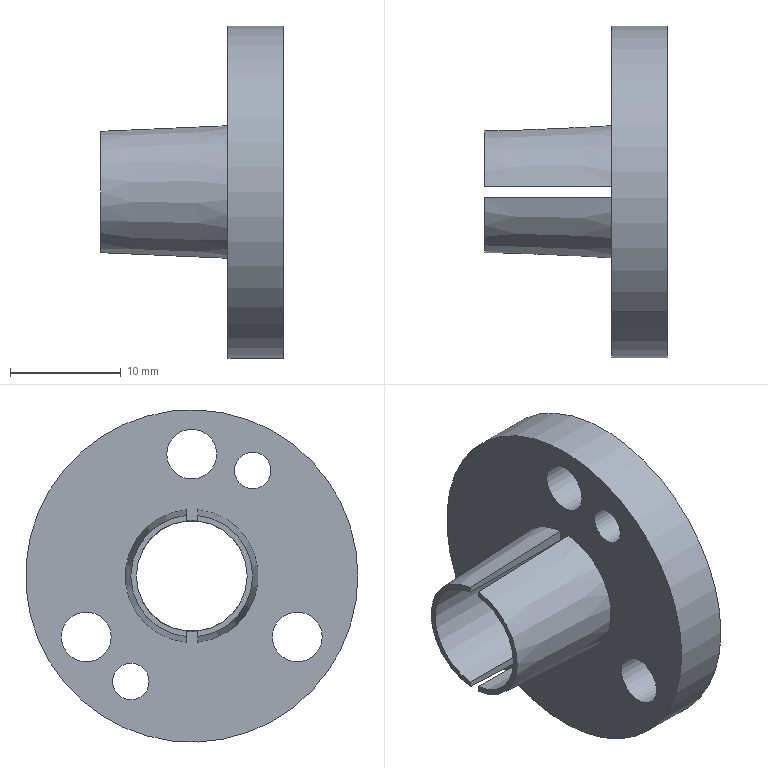Part | NX | features Bushing_5003_015_HTLA24S5M150-E-10 2 | 1 solid | 17 faces | box 16.5 x 30 x 30 mm | volume 3093 mm3 | plane 8 | cylinder 7 | cone 2 | commonest cylinder face diameters 4.5 x3 3.3 x2 10 x1 30 x1
STEP:
#1=CARTESIAN_POINT('',(224.025,119.,-147.));
#2=VERTEX_POINT('',#1);
#3=CARTESIAN_POINT('',(224.025,124.,-147.));
#4=DIRECTION('',(-1.,0.,0.));
#5=DIRECTION('',(0.,-1.,0.));
#6=AXIS2_PLACEMENT_3D('',#3,#4,#5);
#7=CIRCLE('',#6,5.);
#8=EDGE_CURVE('',#2,#2,#7,.T.);
#9=ORIENTED_EDGE('',*,*,#8,.F.);
#10=EDGE_LOOP('',(#9));
#11=FACE_BOUND('',#10,.T.);
#12=CARTESIAN_POINT('',(219.025,123.5,-151.975));
#13=VERTEX_POINT('',#12);
#14=CARTESIAN_POINT('',(219.025,124.5,-151.975));
#15=VERTEX_POINT('',#14);
#16=CARTESIAN_POINT('',(219.025,124.,-147.));
#17=DIRECTION('',(1.,0.,0.));
#18=DIRECTION('',(0.,1.,0.));
#19=AXIS2_PLACEMENT_3D('',#16,#17,#18);
#20=CIRCLE('',#19,5.);
#21=EDGE_CURVE('',#13,#15,#20,.T.);
#22=ORIENTED_EDGE('',*,*,#21,.F.);
#23=CARTESIAN_POINT('',(207.525,123.5,-151.975));
#24=VERTEX_POINT('',#23);
#25=CARTESIAN_POINT('',(207.525,123.5,-151.975));
#26=DIRECTION('',(-1.,0.,0.));
#27=VECTOR('',#26,1000.);
#28=LINE('',#25,#27);
#29=EDGE_CURVE('',#13,#24,#28,.T.);
#30=ORIENTED_EDGE('',*,*,#29,.T.);
#31=CARTESIAN_POINT('',(207.525,123.5,-142.025));
#32=VERTEX_POINT('',#31);
#33=CARTESIAN_POINT('',(207.525,124.,-147.));
#34=DIRECTION('',(-1.,0.,0.));
#35=DIRECTION('',(0.,-1.,0.));
#36=AXIS2_PLACEMENT_3D('',#33,#34,#35);
#37=CIRCLE('',#36,5.);
#38=EDGE_CURVE('',#24,#32,#37,.T.);
#39=ORIENTED_EDGE('',*,*,#38,.T.);
#40=CARTESIAN_POINT('',(219.025,123.5,-142.025));
#41=VERTEX_POINT('',#40);
#42=CARTESIAN_POINT('',(207.525,123.5,-142.025));
#43=DIRECTION('',(-1.,0.,0.));
#44=VECTOR('',#43,1000.);
#45=LINE('',#42,#44);
#46=EDGE_CURVE('',#32,#41,#45,.F.);
#47=ORIENTED_EDGE('',*,*,#46,.T.);
#48=CARTESIAN_POINT('',(219.025,124.5,-142.025));
#49=VERTEX_POINT('',#48);
#50=CARTESIAN_POINT('',(219.025,124.,-147.));
#51=DIRECTION('',(1.,0.,0.));
#52=DIRECTION('',(0.,1.,0.));
#53=AXIS2_PLACEMENT_3D('',#50,#51,#52);
#54=CIRCLE('',#53,5.);
#55=EDGE_CURVE('',#49,#41,#54,.T.);
#56=ORIENTED_EDGE('',*,*,#55,.F.);
#57=CARTESIAN_POINT('',(207.525,124.5,-142.025));
#58=VERTEX_POINT('',#57);
#59=CARTESIAN_POINT('',(207.525,124.5,-142.025));
#60=DIRECTION('',(-1.,0.,0.));
#61=VECTOR('',#60,1000.);
#62=LINE('',#59,#61);
#63=EDGE_CURVE('',#58,#49,#62,.F.);
#64=ORIENTED_EDGE('',*,*,#63,.F.);
#65=CARTESIAN_POINT('',(207.525,124.5,-151.975));
#66=VERTEX_POINT('',#65);
#67=CARTESIAN_POINT('',(207.525,124.,-147.));
#68=DIRECTION('',(-1.,0.,0.));
#69=DIRECTION('',(0.,-1.,0.));
#70=AXIS2_PLACEMENT_3D('',#67,#68,#69);
#71=CIRCLE('',#70,5.);
#72=EDGE_CURVE('',#58,#66,#71,.T.);
#73=ORIENTED_EDGE('',*,*,#72,.T.);
#74=CARTESIAN_POINT('',(207.525,124.5,-151.975));
#75=DIRECTION('',(-1.,0.,0.));
#76=VECTOR('',#75,1000.);
#77=LINE('',#74,#76);
#78=EDGE_CURVE('',#15,#66,#77,.T.);
#79=ORIENTED_EDGE('',*,*,#78,.F.);
#80=EDGE_LOOP('',(#22,#30,#39,#47,#56,#64,#73,#79));
#81=FACE_BOUND('',#80,.T.);
#82=CARTESIAN_POINT('',(207.525,124.,-147.));
#83=DIRECTION('',(-1.,0.,0.));
#84=DIRECTION('',(0.,-1.,0.));
#85=AXIS2_PLACEMENT_3D('',#82,#83,#84);
#86=CYLINDRICAL_SURFACE('',#85,5.);
#87=ADVANCED_FACE('',(#11,#81),#86,.F.);
#88=CARTESIAN_POINT('',(207.525,123.5,-152.477));
#89=VERTEX_POINT('',#88);
#90=CARTESIAN_POINT('',(207.525,123.5,-141.523));
#91=VERTEX_POINT('',#90);
#92=CARTESIAN_POINT('',(207.525,124.,-147.));
#93=DIRECTION('',(-1.,0.,0.));
#94=DIRECTION('',(0.,-1.,0.));
#95=AXIS2_PLACEMENT_3D('',#92,#93,#94);
#96=CIRCLE('',#95,5.5);
#97=EDGE_CURVE('',#89,#91,#96,.T.);
#98=ORIENTED_EDGE('',*,*,#97,.T.);
#99=CARTESIAN_POINT('',(207.525,123.5,-140.996));
#100=DIRECTION('',(0.,0.,1.));
#101=VECTOR('',#100,1000.);
#102=LINE('',#99,#101);
#103=EDGE_CURVE('',#32,#91,#102,.T.);
#104=ORIENTED_EDGE('',*,*,#103,.F.);
#105=ORIENTED_EDGE('',*,*,#38,.F.);
#106=CARTESIAN_POINT('',(207.525,123.5,-140.996));
#107=DIRECTION('',(0.,0.,1.));
#108=VECTOR('',#107,1000.);
#109=LINE('',#106,#108);
#110=EDGE_CURVE('',#89,#24,#109,.T.);
#111=ORIENTED_EDGE('',*,*,#110,.F.);
#112=EDGE_LOOP('',(#98,#104,#105,#111));
#113=FACE_BOUND('',#112,.T.);
#114=CARTESIAN_POINT('',(207.525,124.,-142.));
#115=DIRECTION('',(-1.,0.,0.));
#116=DIRECTION('',(0.,-1.,0.));
#117=AXIS2_PLACEMENT_3D('',#114,#115,#116);
#118=PLANE('',#117);
#119=ADVANCED_FACE('',(#113),#118,.T.);
#120=ORIENTED_EDGE('',*,*,#97,.F.);
#121=CARTESIAN_POINT('',(219.025,123.5,-152.983));
#122=VERTEX_POINT('',#121);
#123=CARTESIAN_POINT('',(219.025,123.5,-152.983));
#124=CARTESIAN_POINT('',(215.192,123.5,-152.815));
#125=CARTESIAN_POINT('',(211.358,123.5,-152.646));
#126=CARTESIAN_POINT('',(207.525,123.5,-152.477));
#127=B_SPLINE_CURVE_WITH_KNOTS('',3,(#123,#124,#125,#126),.UNSPECIFIED.,.F.,.F.,(4,4),(0.009877,0.02139),.UNSPECIFIED.);
#128=EDGE_CURVE('',#89,#122,#127,.F.);
#129=ORIENTED_EDGE('',*,*,#128,.T.);
#130=CARTESIAN_POINT('',(219.025,123.5,-141.017));
#131=VERTEX_POINT('',#130);
#132=CARTESIAN_POINT('',(219.025,124.,-147.));
#133=DIRECTION('',(-1.,0.,0.));
#134=DIRECTION('',(0.,-1.,0.));
#135=AXIS2_PLACEMENT_3D('',#132,#133,#134);
#136=CIRCLE('',#135,6.004);
#137=EDGE_CURVE('',#122,#131,#136,.T.);
#138=ORIENTED_EDGE('',*,*,#137,.T.);
#139=CARTESIAN_POINT('',(219.025,123.5,-141.017));
#140=CARTESIAN_POINT('',(215.192,123.5,-141.185));
#141=CARTESIAN_POINT('',(211.358,123.5,-141.354));
#142=CARTESIAN_POINT('',(207.525,123.5,-141.523));
#143=B_SPLINE_CURVE_WITH_KNOTS('',3,(#139,#140,#141,#142),.UNSPECIFIED.,.F.,.F.,(4,4),(0.009877,0.02139),.UNSPECIFIED.);
#144=EDGE_CURVE('',#131,#91,#143,.T.);
#145=ORIENTED_EDGE('',*,*,#144,.T.);
#146=EDGE_LOOP('',(#120,#129,#138,#145));
#147=FACE_BOUND('',#146,.T.);
#148=CARTESIAN_POINT('',(207.525,124.,-147.));
#149=DIRECTION('',(1.,0.,0.));
#150=DIRECTION('',(0.,1.,0.));
#151=AXIS2_PLACEMENT_3D('',#148,#149,#150);
#152=CONICAL_SURFACE('',#151,5.5,0.0438);
#153=ADVANCED_FACE('',(#147),#152,.T.);
#154=CARTESIAN_POINT('',(224.025,109.,-147.));
#155=VERTEX_POINT('',#154);
#156=CARTESIAN_POINT('',(224.025,124.,-147.));
#157=DIRECTION('',(-1.,0.,0.));
#158=DIRECTION('',(0.,-1.,0.));
#159=AXIS2_PLACEMENT_3D('',#156,#157,#158);
#160=CIRCLE('',#159,15.);
#161=EDGE_CURVE('',#155,#155,#160,.T.);
#162=ORIENTED_EDGE('',*,*,#161,.T.);
#163=EDGE_LOOP('',(#162));
#164=FACE_BOUND('',#163,.T.);
#165=CARTESIAN_POINT('',(219.025,109.,-147.));
#166=VERTEX_POINT('',#165);
#167=CARTESIAN_POINT('',(219.025,124.,-147.));
#168=DIRECTION('',(-1.,0.,0.));
#169=DIRECTION('',(0.,-1.,0.));
#170=AXIS2_PLACEMENT_3D('',#167,#168,#169);
#171=CIRCLE('',#170,15.);
#172=EDGE_CURVE('',#166,#166,#171,.T.);
#173=ORIENTED_EDGE('',*,*,#172,.F.);
#174=EDGE_LOOP('',(#173));
#175=FACE_BOUND('',#174,.T.);
#176=CARTESIAN_POINT('',(207.525,124.,-147.));
#177=DIRECTION('',(-1.,0.,0.));
#178=DIRECTION('',(0.,-1.,0.));
#179=AXIS2_PLACEMENT_3D('',#176,#177,#178);
#180=CYLINDRICAL_SURFACE('',#179,15.);
#181=ADVANCED_FACE('',(#164,#175),#180,.T.);
#182=CARTESIAN_POINT('',(224.025,120.15,-137.474));
#183=VERTEX_POINT('',#182);
#184=CARTESIAN_POINT('',(224.025,118.5,-137.474));
#185=DIRECTION('',(1.,0.,0.));
#186=DIRECTION('',(0.,1.,0.));
#187=AXIS2_PLACEMENT_3D('',#184,#185,#186);
#188=CIRCLE('',#187,1.65);
#189=EDGE_CURVE('',#183,#183,#188,.T.);
#190=ORIENTED_EDGE('',*,*,#189,.F.);
#191=EDGE_LOOP('',(#190));
#192=FACE_BOUND('',#191,.T.);
#193=CARTESIAN_POINT('',(224.025,131.15,-156.526));
#194=VERTEX_POINT('',#193);
#195=CARTESIAN_POINT('',(224.025,129.5,-156.526));
#196=DIRECTION('',(1.,0.,0.));
#197=DIRECTION('',(0.,1.,0.));
#198=AXIS2_PLACEMENT_3D('',#195,#196,#197);
#199=CIRCLE('',#198,1.65);
#200=EDGE_CURVE('',#194,#194,#199,.T.);
#201=ORIENTED_EDGE('',*,*,#200,.F.);
#202=EDGE_LOOP('',(#201));
#203=FACE_BOUND('',#202,.T.);
#204=CARTESIAN_POINT('',(224.025,126.25,-136.));
#205=VERTEX_POINT('',#204);
#206=CARTESIAN_POINT('',(224.025,124.,-136.));
#207=DIRECTION('',(1.,0.,0.));
#208=DIRECTION('',(0.,1.,0.));
#209=AXIS2_PLACEMENT_3D('',#206,#207,#208);
#210=CIRCLE('',#209,2.25);
#211=EDGE_CURVE('',#205,#205,#210,.T.);
#212=ORIENTED_EDGE('',*,*,#211,.F.);
#213=EDGE_LOOP('',(#212));
#214=FACE_BOUND('',#213,.T.);
#215=CARTESIAN_POINT('',(224.025,135.776,-152.5));
#216=VERTEX_POINT('',#215);
#217=CARTESIAN_POINT('',(224.025,133.526,-152.5));
#218=DIRECTION('',(1.,0.,0.));
#219=DIRECTION('',(0.,1.,0.));
#220=AXIS2_PLACEMENT_3D('',#217,#218,#219);
#221=CIRCLE('',#220,2.25);
#222=EDGE_CURVE('',#216,#216,#221,.T.);
#223=ORIENTED_EDGE('',*,*,#222,.F.);
#224=EDGE_LOOP('',(#223));
#225=FACE_BOUND('',#224,.T.);
#226=CARTESIAN_POINT('',(224.025,116.724,-152.5));
#227=VERTEX_POINT('',#226);
#228=CARTESIAN_POINT('',(224.025,114.474,-152.5));
#229=DIRECTION('',(1.,0.,0.));
#230=DIRECTION('',(0.,1.,0.));
#231=AXIS2_PLACEMENT_3D('',#228,#229,#230);
#232=CIRCLE('',#231,2.25);
#233=EDGE_CURVE('',#227,#227,#232,.T.);
#234=ORIENTED_EDGE('',*,*,#233,.F.);
#235=EDGE_LOOP('',(#234));
#236=FACE_BOUND('',#235,.T.);
#237=ORIENTED_EDGE('',*,*,#8,.T.);
#238=EDGE_LOOP('',(#237));
#239=FACE_BOUND('',#238,.T.);
#240=ORIENTED_EDGE('',*,*,#161,.F.);
#241=EDGE_LOOP('',(#240));
#242=FACE_BOUND('',#241,.T.);
#243=CARTESIAN_POINT('',(224.025,124.,-132.));
#244=DIRECTION('',(1.,0.,0.));
#245=DIRECTION('',(0.,1.,0.));
#246=AXIS2_PLACEMENT_3D('',#243,#244,#245);
#247=PLANE('',#246);
#248=ADVANCED_FACE('',(#192,#203,#214,#225,#236,#239,#242),#247,.T.);
#249=CARTESIAN_POINT('',(207.525,124.5,-141.523));
#250=VERTEX_POINT('',#249);
#251=CARTESIAN_POINT('',(207.525,124.5,-140.996));
#252=DIRECTION('',(0.,0.,1.));
#253=VECTOR('',#252,1000.);
#254=LINE('',#251,#253);
#255=EDGE_CURVE('',#58,#250,#254,.T.);
#256=ORIENTED_EDGE('',*,*,#255,.T.);
#257=CARTESIAN_POINT('',(207.525,124.5,-152.477));
#258=VERTEX_POINT('',#257);
#259=CARTESIAN_POINT('',(207.525,124.,-147.));
#260=DIRECTION('',(-1.,0.,0.));
#261=DIRECTION('',(0.,-1.,0.));
#262=AXIS2_PLACEMENT_3D('',#259,#260,#261);
#263=CIRCLE('',#262,5.5);
#264=EDGE_CURVE('',#250,#258,#263,.T.);
#265=ORIENTED_EDGE('',*,*,#264,.T.);
#266=CARTESIAN_POINT('',(207.525,124.5,-140.996));
#267=DIRECTION('',(0.,0.,1.));
#268=VECTOR('',#267,1000.);
#269=LINE('',#266,#268);
#270=EDGE_CURVE('',#258,#66,#269,.T.);
#271=ORIENTED_EDGE('',*,*,#270,.T.);
#272=ORIENTED_EDGE('',*,*,#72,.F.);
#273=EDGE_LOOP('',(#256,#265,#271,#272));
#274=FACE_BOUND('',#273,.T.);
#275=CARTESIAN_POINT('',(207.525,124.,-142.));
#276=DIRECTION('',(-1.,0.,0.));
#277=DIRECTION('',(0.,-1.,0.));
#278=AXIS2_PLACEMENT_3D('',#275,#276,#277);
#279=PLANE('',#278);
#280=ADVANCED_FACE('',(#274),#279,.T.);
#281=CARTESIAN_POINT('',(219.025,124.5,-152.983));
#282=VERTEX_POINT('',#281);
#283=CARTESIAN_POINT('',(219.025,124.5,-152.983));
#284=CARTESIAN_POINT('',(215.192,124.5,-152.815));
#285=CARTESIAN_POINT('',(211.358,124.5,-152.646));
#286=CARTESIAN_POINT('',(207.525,124.5,-152.477));
#287=B_SPLINE_CURVE_WITH_KNOTS('',3,(#283,#284,#285,#286),.UNSPECIFIED.,.F.,.F.,(4,4),(0.009877,0.02139),.UNSPECIFIED.);
#288=EDGE_CURVE('',#258,#282,#287,.F.);
#289=ORIENTED_EDGE('',*,*,#288,.F.);
#290=ORIENTED_EDGE('',*,*,#264,.F.);
#291=CARTESIAN_POINT('',(219.025,124.5,-141.017));
#292=VERTEX_POINT('',#291);
#293=CARTESIAN_POINT('',(219.025,124.5,-141.017));
#294=CARTESIAN_POINT('',(215.192,124.5,-141.185));
#295=CARTESIAN_POINT('',(211.358,124.5,-141.354));
#296=CARTESIAN_POINT('',(207.525,124.5,-141.523));
#297=B_SPLINE_CURVE_WITH_KNOTS('',3,(#293,#294,#295,#296),.UNSPECIFIED.,.F.,.F.,(4,4),(0.009877,0.02139),.UNSPECIFIED.);
#298=EDGE_CURVE('',#292,#250,#297,.T.);
#299=ORIENTED_EDGE('',*,*,#298,.F.);
#300=CARTESIAN_POINT('',(219.025,124.,-147.));
#301=DIRECTION('',(-1.,0.,0.));
#302=DIRECTION('',(0.,-1.,0.));
#303=AXIS2_PLACEMENT_3D('',#300,#301,#302);
#304=CIRCLE('',#303,6.004);
#305=EDGE_CURVE('',#292,#282,#304,.T.);
#306=ORIENTED_EDGE('',*,*,#305,.T.);
#307=EDGE_LOOP('',(#289,#290,#299,#306));
#308=FACE_BOUND('',#307,.T.);
#309=CARTESIAN_POINT('',(207.525,124.,-147.));
#310=DIRECTION('',(1.,0.,0.));
#311=DIRECTION('',(0.,1.,0.));
#312=AXIS2_PLACEMENT_3D('',#309,#310,#311);
#313=CONICAL_SURFACE('',#312,5.5,0.0438);
#314=ADVANCED_FACE('',(#308),#313,.T.);
#315=CARTESIAN_POINT('',(219.025,116.85,-137.474));
#316=VERTEX_POINT('',#315);
#317=CARTESIAN_POINT('',(219.025,118.5,-137.474));
#318=DIRECTION('',(-1.,0.,0.));
#319=DIRECTION('',(0.,-1.,0.));
#320=AXIS2_PLACEMENT_3D('',#317,#318,#319);
#321=CIRCLE('',#320,1.65);
#322=EDGE_CURVE('',#316,#316,#321,.T.);
#323=ORIENTED_EDGE('',*,*,#322,.F.);
#324=EDGE_LOOP('',(#323));
#325=FACE_BOUND('',#324,.T.);
#326=CARTESIAN_POINT('',(219.025,127.85,-156.526));
#327=VERTEX_POINT('',#326);
#328=CARTESIAN_POINT('',(219.025,129.5,-156.526));
#329=DIRECTION('',(-1.,0.,0.));
#330=DIRECTION('',(0.,-1.,0.));
#331=AXIS2_PLACEMENT_3D('',#328,#329,#330);
#332=CIRCLE('',#331,1.65);
#333=EDGE_CURVE('',#327,#327,#332,.T.);
#334=ORIENTED_EDGE('',*,*,#333,.F.);
#335=EDGE_LOOP('',(#334));
#336=FACE_BOUND('',#335,.T.);
#337=CARTESIAN_POINT('',(219.025,121.75,-136.));
#338=VERTEX_POINT('',#337);
#339=CARTESIAN_POINT('',(219.025,124.,-136.));
#340=DIRECTION('',(-1.,0.,0.));
#341=DIRECTION('',(0.,-1.,0.));
#342=AXIS2_PLACEMENT_3D('',#339,#340,#341);
#343=CIRCLE('',#342,2.25);
#344=EDGE_CURVE('',#338,#338,#343,.T.);
#345=ORIENTED_EDGE('',*,*,#344,.F.);
#346=EDGE_LOOP('',(#345));
#347=FACE_BOUND('',#346,.T.);
#348=CARTESIAN_POINT('',(219.025,131.276,-152.5));
#349=VERTEX_POINT('',#348);
#350=CARTESIAN_POINT('',(219.025,133.526,-152.5));
#351=DIRECTION('',(-1.,0.,0.));
#352=DIRECTION('',(0.,-1.,0.));
#353=AXIS2_PLACEMENT_3D('',#350,#351,#352);
#354=CIRCLE('',#353,2.25);
#355=EDGE_CURVE('',#349,#349,#354,.T.);
#356=ORIENTED_EDGE('',*,*,#355,.F.);
#357=EDGE_LOOP('',(#356));
#358=FACE_BOUND('',#357,.T.);
#359=CARTESIAN_POINT('',(219.025,112.224,-152.5));
#360=VERTEX_POINT('',#359);
#361=CARTESIAN_POINT('',(219.025,114.474,-152.5));
#362=DIRECTION('',(-1.,0.,0.));
#363=DIRECTION('',(0.,-1.,0.));
#364=AXIS2_PLACEMENT_3D('',#361,#362,#363);
#365=CIRCLE('',#364,2.25);
#366=EDGE_CURVE('',#360,#360,#365,.T.);
#367=ORIENTED_EDGE('',*,*,#366,.F.);
#368=EDGE_LOOP('',(#367));
#369=FACE_BOUND('',#368,.T.);
#370=ORIENTED_EDGE('',*,*,#305,.F.);
#371=CARTESIAN_POINT('',(219.025,124.5,-140.996));
#372=DIRECTION('',(0.,0.,-1.));
#373=VECTOR('',#372,1000.);
#374=LINE('',#371,#373);
#375=EDGE_CURVE('',#292,#49,#374,.T.);
#376=ORIENTED_EDGE('',*,*,#375,.T.);
#377=ORIENTED_EDGE('',*,*,#55,.T.);
#378=CARTESIAN_POINT('',(219.025,123.5,-140.996));
#379=DIRECTION('',(0.,0.,-1.));
#380=VECTOR('',#379,1000.);
#381=LINE('',#378,#380);
#382=EDGE_CURVE('',#131,#41,#381,.T.);
#383=ORIENTED_EDGE('',*,*,#382,.F.);
#384=ORIENTED_EDGE('',*,*,#137,.F.);
#385=CARTESIAN_POINT('',(219.025,123.5,-140.996));
#386=DIRECTION('',(0.,0.,-1.));
#387=VECTOR('',#386,1000.);
#388=LINE('',#385,#387);
#389=EDGE_CURVE('',#13,#122,#388,.T.);
#390=ORIENTED_EDGE('',*,*,#389,.F.);
#391=ORIENTED_EDGE('',*,*,#21,.T.);
#392=CARTESIAN_POINT('',(219.025,124.5,-140.996));
#393=DIRECTION('',(0.,0.,-1.));
#394=VECTOR('',#393,1000.);
#395=LINE('',#392,#394);
#396=EDGE_CURVE('',#15,#282,#395,.T.);
#397=ORIENTED_EDGE('',*,*,#396,.T.);
#398=EDGE_LOOP('',(#370,#376,#377,#383,#384,#390,#391,#397));
#399=FACE_BOUND('',#398,.T.);
#400=ORIENTED_EDGE('',*,*,#172,.T.);
#401=EDGE_LOOP('',(#400));
#402=FACE_BOUND('',#401,.T.);
#403=CARTESIAN_POINT('',(219.025,124.,-140.996));
#404=DIRECTION('',(-1.,0.,0.));
#405=DIRECTION('',(0.,-1.,0.));
#406=AXIS2_PLACEMENT_3D('',#403,#404,#405);
#407=PLANE('',#406);
#408=ADVANCED_FACE('',(#325,#336,#347,#358,#369,#399,#402),#407,.T.);
#409=ORIENTED_EDGE('',*,*,#103,.T.);
#410=ORIENTED_EDGE('',*,*,#144,.F.);
#411=ORIENTED_EDGE('',*,*,#382,.T.);
#412=ORIENTED_EDGE('',*,*,#46,.F.);
#413=EDGE_LOOP('',(#409,#410,#411,#412));
#414=FACE_BOUND('',#413,.T.);
#415=CARTESIAN_POINT('',(224.025,123.5,-147.));
#416=DIRECTION('',(0.,1.,0.));
#417=DIRECTION('',(-1.,0.,0.));
#418=AXIS2_PLACEMENT_3D('',#415,#416,#417);
#419=PLANE('',#418);
#420=ADVANCED_FACE('',(#414),#419,.T.);
#421=ORIENTED_EDGE('',*,*,#63,.T.);
#422=ORIENTED_EDGE('',*,*,#375,.F.);
#423=ORIENTED_EDGE('',*,*,#298,.T.);
#424=ORIENTED_EDGE('',*,*,#255,.F.);
#425=EDGE_LOOP('',(#421,#422,#423,#424));
#426=FACE_BOUND('',#425,.T.);
#427=CARTESIAN_POINT('',(224.025,124.5,-147.));
#428=DIRECTION('',(0.,1.,0.));
#429=DIRECTION('',(-1.,0.,0.));
#430=AXIS2_PLACEMENT_3D('',#427,#428,#429);
#431=PLANE('',#430);
#432=ADVANCED_FACE('',(#426),#431,.F.);
#433=ORIENTED_EDGE('',*,*,#389,.T.);
#434=ORIENTED_EDGE('',*,*,#128,.F.);
#435=ORIENTED_EDGE('',*,*,#110,.T.);
#436=ORIENTED_EDGE('',*,*,#29,.F.);
#437=EDGE_LOOP('',(#433,#434,#435,#436));
#438=FACE_BOUND('',#437,.T.);
#439=CARTESIAN_POINT('',(224.025,123.5,-147.));
#440=DIRECTION('',(0.,1.,0.));
#441=DIRECTION('',(-1.,0.,0.));
#442=AXIS2_PLACEMENT_3D('',#439,#440,#441);
#443=PLANE('',#442);
#444=ADVANCED_FACE('',(#438),#443,.T.);
#445=ORIENTED_EDGE('',*,*,#78,.T.);
#446=ORIENTED_EDGE('',*,*,#270,.F.);
#447=ORIENTED_EDGE('',*,*,#288,.T.);
#448=ORIENTED_EDGE('',*,*,#396,.F.);
#449=EDGE_LOOP('',(#445,#446,#447,#448));
#450=FACE_BOUND('',#449,.T.);
#451=CARTESIAN_POINT('',(224.025,124.5,-147.));
#452=DIRECTION('',(0.,1.,0.));
#453=DIRECTION('',(-1.,0.,0.));
#454=AXIS2_PLACEMENT_3D('',#451,#452,#453);
#455=PLANE('',#454);
#456=ADVANCED_FACE('',(#450),#455,.F.);
#457=ORIENTED_EDGE('',*,*,#366,.T.);
#458=EDGE_LOOP('',(#457));
#459=FACE_BOUND('',#458,.T.);
#460=ORIENTED_EDGE('',*,*,#233,.T.);
#461=EDGE_LOOP('',(#460));
#462=FACE_BOUND('',#461,.T.);
#463=CARTESIAN_POINT('',(224.025,114.474,-152.5));
#464=DIRECTION('',(1.,0.,0.));
#465=DIRECTION('',(0.,1.,0.));
#466=AXIS2_PLACEMENT_3D('',#463,#464,#465);
#467=CYLINDRICAL_SURFACE('',#466,2.25);
#468=ADVANCED_FACE('',(#459,#462),#467,.F.);
#469=ORIENTED_EDGE('',*,*,#355,.T.);
#470=EDGE_LOOP('',(#469));
#471=FACE_BOUND('',#470,.T.);
#472=ORIENTED_EDGE('',*,*,#222,.T.);
#473=EDGE_LOOP('',(#472));
#474=FACE_BOUND('',#473,.T.);
#475=CARTESIAN_POINT('',(224.025,133.526,-152.5));
#476=DIRECTION('',(1.,0.,0.));
#477=DIRECTION('',(0.,1.,0.));
#478=AXIS2_PLACEMENT_3D('',#475,#476,#477);
#479=CYLINDRICAL_SURFACE('',#478,2.25);
#480=ADVANCED_FACE('',(#471,#474),#479,.F.);
#481=ORIENTED_EDGE('',*,*,#344,.T.);
#482=EDGE_LOOP('',(#481));
#483=FACE_BOUND('',#482,.T.);
#484=ORIENTED_EDGE('',*,*,#211,.T.);
#485=EDGE_LOOP('',(#484));
#486=FACE_BOUND('',#485,.T.);
#487=CARTESIAN_POINT('',(224.025,124.,-136.));
#488=DIRECTION('',(1.,0.,0.));
#489=DIRECTION('',(0.,1.,0.));
#490=AXIS2_PLACEMENT_3D('',#487,#488,#489);
#491=CYLINDRICAL_SURFACE('',#490,2.25);
#492=ADVANCED_FACE('',(#483,#486),#491,.F.);
#493=ORIENTED_EDGE('',*,*,#333,.T.);
#494=EDGE_LOOP('',(#493));
#495=FACE_BOUND('',#494,.T.);
#496=ORIENTED_EDGE('',*,*,#200,.T.);
#497=EDGE_LOOP('',(#496));
#498=FACE_BOUND('',#497,.T.);
#499=CARTESIAN_POINT('',(224.025,129.5,-156.526));
#500=DIRECTION('',(1.,0.,0.));
#501=DIRECTION('',(0.,1.,0.));
#502=AXIS2_PLACEMENT_3D('',#499,#500,#501);
#503=CYLINDRICAL_SURFACE('',#502,1.65);
#504=ADVANCED_FACE('',(#495,#498),#503,.F.);
#505=ORIENTED_EDGE('',*,*,#322,.T.);
#506=EDGE_LOOP('',(#505));
#507=FACE_BOUND('',#506,.T.);
#508=ORIENTED_EDGE('',*,*,#189,.T.);
#509=EDGE_LOOP('',(#508));
#510=FACE_BOUND('',#509,.T.);
#511=CARTESIAN_POINT('',(224.025,118.5,-137.474));
#512=DIRECTION('',(1.,0.,0.));
#513=DIRECTION('',(0.,1.,0.));
#514=AXIS2_PLACEMENT_3D('',#511,#512,#513);
#515=CYLINDRICAL_SURFACE('',#514,1.65);
#516=ADVANCED_FACE('',(#507,#510),#515,.F.);
#517=CLOSED_SHELL('',(#87,#119,#153,#181,#248,#280,#314,#408,#420,#432,#444,#456,#468,#480,#492,#504,#516));
#518=MANIFOLD_SOLID_BREP('',#517);
#519=(LENGTH_UNIT()NAMED_UNIT(*)SI_UNIT(.MILLI.,.METRE.));
#520=UNCERTAINTY_MEASURE_WITH_UNIT(LENGTH_MEASURE(0.0508),#519,'','');
#521=(NAMED_UNIT(*)PLANE_ANGLE_UNIT()SI_UNIT($,.RADIAN.));
#522=(NAMED_UNIT(*)SI_UNIT($,.STERADIAN.)SOLID_ANGLE_UNIT());
#523=(GEOMETRIC_REPRESENTATION_CONTEXT(3)GLOBAL_UNCERTAINTY_ASSIGNED_CONTEXT((#520))GLOBAL_UNIT_ASSIGNED_CONTEXT((#519,#521,#522))REPRESENTATION_CONTEXT('',''));
#524=ADVANCED_BREP_SHAPE_REPRESENTATION('',(#518),#523);